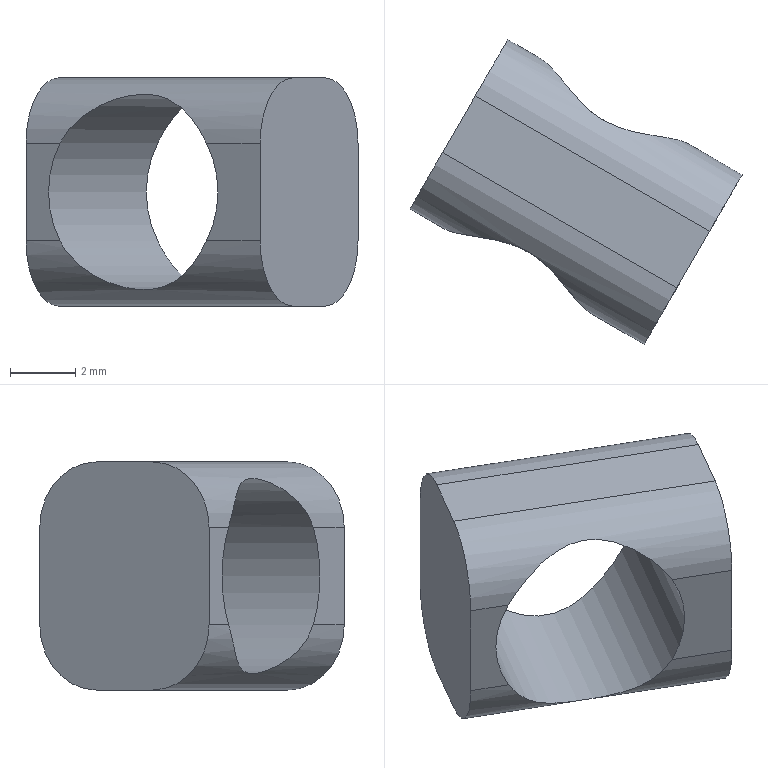Part | STEP file | 1 solid | 13 faces | box 10.188 x 9.346 x 7 mm | volume 153.66 mm3 | plane 8 | cylinder 5 | commonest cylinder face diameters 4 x4 6 x1
STEP:
#1=CARTESIAN_POINT('',(39.484,-2.012,-6.75));
#2=VERTEX_POINT('',#1);
#3=CARTESIAN_POINT('',(40.484,-0.2795,-4.75));
#4=VERTEX_POINT('',#3);
#5=CARTESIAN_POINT('',(40.484,-0.2795,-6.75));
#6=DIRECTION('',(-0.866,0.5,0.));
#7=DIRECTION('',(-0.5,-0.866,0.));
#8=AXIS2_PLACEMENT_3D('',#5,#6,#7);
#9=CIRCLE('',#8,2.);
#10=EDGE_CURVE('',#2,#4,#9,.T.);
#11=ORIENTED_EDGE('',*,*,#10,.T.);
#12=CARTESIAN_POINT('',(41.484,1.453,-4.75));
#13=VERTEX_POINT('',#12);
#14=CARTESIAN_POINT('',(40.484,-0.2795,-4.75));
#15=DIRECTION('',(0.5,0.866,0.));
#16=VECTOR('',#15,1.);
#17=LINE('',#14,#16);
#18=EDGE_CURVE('',#4,#13,#17,.T.);
#19=ORIENTED_EDGE('',*,*,#18,.T.);
#20=CARTESIAN_POINT('',(42.484,3.185,-6.75));
#21=VERTEX_POINT('',#20);
#22=CARTESIAN_POINT('',(41.484,1.453,-6.75));
#23=DIRECTION('',(-0.866,0.5,0.));
#24=DIRECTION('',(0.,0.,1.));
#25=AXIS2_PLACEMENT_3D('',#22,#23,#24);
#26=CIRCLE('',#25,2.);
#27=EDGE_CURVE('',#13,#21,#26,.T.);
#28=ORIENTED_EDGE('',*,*,#27,.T.);
#29=CARTESIAN_POINT('',(42.484,3.185,-9.75));
#30=VERTEX_POINT('',#29);
#31=CARTESIAN_POINT('',(42.484,3.185,-6.75));
#32=DIRECTION('',(0.,0.,-1.));
#33=VECTOR('',#32,1.);
#34=LINE('',#31,#33);
#35=EDGE_CURVE('',#21,#30,#34,.T.);
#36=ORIENTED_EDGE('',*,*,#35,.T.);
#37=CARTESIAN_POINT('',(41.484,1.453,-11.75));
#38=VERTEX_POINT('',#37);
#39=CARTESIAN_POINT('',(41.484,1.453,-9.75));
#40=DIRECTION('',(-0.866,0.5,0.));
#41=DIRECTION('',(0.5,0.866,0.));
#42=AXIS2_PLACEMENT_3D('',#39,#40,#41);
#43=CIRCLE('',#42,2.);
#44=EDGE_CURVE('',#30,#38,#43,.T.);
#45=ORIENTED_EDGE('',*,*,#44,.T.);
#46=CARTESIAN_POINT('',(40.484,-0.2795,-11.75));
#47=VERTEX_POINT('',#46);
#48=CARTESIAN_POINT('',(41.484,1.453,-11.75));
#49=DIRECTION('',(-0.5,-0.866,0.));
#50=VECTOR('',#49,1.);
#51=LINE('',#48,#50);
#52=EDGE_CURVE('',#38,#47,#51,.T.);
#53=ORIENTED_EDGE('',*,*,#52,.T.);
#54=CARTESIAN_POINT('',(39.484,-2.012,-9.75));
#55=VERTEX_POINT('',#54);
#56=CARTESIAN_POINT('',(40.484,-0.2795,-9.75));
#57=DIRECTION('',(-0.866,0.5,0.));
#58=DIRECTION('',(0.,0.,-1.));
#59=AXIS2_PLACEMENT_3D('',#56,#57,#58);
#60=CIRCLE('',#59,2.);
#61=EDGE_CURVE('',#47,#55,#60,.T.);
#62=ORIENTED_EDGE('',*,*,#61,.T.);
#63=CARTESIAN_POINT('',(39.484,-2.012,-9.75));
#64=DIRECTION('',(0.,0.,1.));
#65=VECTOR('',#64,1.);
#66=LINE('',#63,#65);
#67=EDGE_CURVE('',#55,#2,#66,.T.);
#68=ORIENTED_EDGE('',*,*,#67,.T.);
#69=EDGE_LOOP('',(#11,#19,#28,#36,#45,#53,#62,#68));
#70=FACE_BOUND('',#69,.T.);
#71=CARTESIAN_POINT('',(40.984,0.5865,-8.25));
#72=DIRECTION('',(0.866,-0.5,0.));
#73=DIRECTION('',(0.,0.,-1.));
#74=AXIS2_PLACEMENT_3D('',#71,#72,#73);
#75=PLANE('',#74);
#76=ADVANCED_FACE('',(#70),#75,.F.);
#77=ORIENTED_EDGE('',*,*,#67,.F.);
#78=CARTESIAN_POINT('',(40.525,-2.613,-9.75));
#79=VERTEX_POINT('',#78);
#80=CARTESIAN_POINT('',(40.525,-2.613,-9.75));
#81=DIRECTION('',(-0.866,0.5,0.));
#82=VECTOR('',#81,1.);
#83=LINE('',#80,#82);
#84=EDGE_CURVE('',#79,#55,#83,.T.);
#85=ORIENTED_EDGE('',*,*,#84,.F.);
#86=CARTESIAN_POINT('',(40.525,-2.613,-6.75));
#87=VERTEX_POINT('',#86);
#88=CARTESIAN_POINT('',(42.775,-3.912,-8.25));
#89=DIRECTION('',(0.5,0.866,0.));
#90=DIRECTION('',(-0.75,0.433,-0.5));
#91=AXIS2_PLACEMENT_3D('',#88,#89,#90);
#92=CIRCLE('',#91,3.);
#93=EDGE_CURVE('',#79,#87,#92,.T.);
#94=ORIENTED_EDGE('',*,*,#93,.T.);
#95=CARTESIAN_POINT('',(39.484,-2.012,-6.75));
#96=DIRECTION('',(0.866,-0.5,0.));
#97=VECTOR('',#96,1.);
#98=LINE('',#95,#97);
#99=EDGE_CURVE('',#2,#87,#98,.T.);
#100=ORIENTED_EDGE('',*,*,#99,.F.);
#101=EDGE_LOOP('',(#77,#85,#94,#100));
#102=FACE_BOUND('',#101,.T.);
#103=CARTESIAN_POINT('',(39.484,-2.012,-6.75));
#104=DIRECTION('',(-0.5,-0.866,0.));
#105=DIRECTION('',(-0.866,0.5,0.));
#106=AXIS2_PLACEMENT_3D('',#103,#104,#105);
#107=PLANE('',#106);
#108=ADVANCED_FACE('',(#102),#107,.T.);
#109=CARTESIAN_POINT('',(47.672,-4.429,-4.75));
#110=VERTEX_POINT('',#109);
#111=CARTESIAN_POINT('',(46.672,-6.162,-6.75));
#112=VERTEX_POINT('',#111);
#113=CARTESIAN_POINT('',(47.672,-4.429,-6.75));
#114=DIRECTION('',(0.866,-0.5,0.));
#115=DIRECTION('',(0.,0.,1.));
#116=AXIS2_PLACEMENT_3D('',#113,#114,#115);
#117=CIRCLE('',#116,2.);
#118=EDGE_CURVE('',#110,#112,#117,.T.);
#119=ORIENTED_EDGE('',*,*,#118,.F.);
#120=CARTESIAN_POINT('',(47.672,-4.429,-4.75));
#121=DIRECTION('',(-0.866,0.5,0.));
#122=VECTOR('',#121,1.);
#123=LINE('',#120,#122);
#124=EDGE_CURVE('',#110,#4,#123,.T.);
#125=ORIENTED_EDGE('',*,*,#124,.T.);
#126=ORIENTED_EDGE('',*,*,#10,.F.);
#127=ORIENTED_EDGE('',*,*,#99,.T.);
#128=CARTESIAN_POINT('',(43.114,-3.325,-5.25));
#129=VERTEX_POINT('',#128);
#130=CARTESIAN_POINT('',(40.525,-2.613,-6.75));
#131=CARTESIAN_POINT('',(40.535,-2.618,-6.731));
#132=CARTESIAN_POINT('',(40.555,-2.629,-6.692));
#133=CARTESIAN_POINT('',(40.587,-2.645,-6.635));
#134=CARTESIAN_POINT('',(40.621,-2.66,-6.578));
#135=CARTESIAN_POINT('',(40.657,-2.674,-6.523));
#136=CARTESIAN_POINT('',(40.694,-2.687,-6.469));
#137=CARTESIAN_POINT('',(40.733,-2.7,-6.415));
#138=CARTESIAN_POINT('',(40.774,-2.713,-6.363));
#139=CARTESIAN_POINT('',(40.816,-2.725,-6.311));
#140=CARTESIAN_POINT('',(40.861,-2.736,-6.26));
#141=CARTESIAN_POINT('',(40.907,-2.748,-6.209));
#142=CARTESIAN_POINT('',(40.956,-2.758,-6.16));
#143=CARTESIAN_POINT('',(41.006,-2.769,-6.111));
#144=CARTESIAN_POINT('',(41.058,-2.78,-6.062));
#145=CARTESIAN_POINT('',(41.112,-2.79,-6.015));
#146=CARTESIAN_POINT('',(41.167,-2.8,-5.968));
#147=CARTESIAN_POINT('',(41.224,-2.81,-5.923));
#148=CARTESIAN_POINT('',(41.282,-2.82,-5.879));
#149=CARTESIAN_POINT('',(41.342,-2.829,-5.837));
#150=CARTESIAN_POINT('',(41.402,-2.839,-5.796));
#151=CARTESIAN_POINT('',(41.462,-2.849,-5.756));
#152=CARTESIAN_POINT('',(41.523,-2.858,-5.719));
#153=CARTESIAN_POINT('',(41.584,-2.868,-5.683));
#154=CARTESIAN_POINT('',(41.645,-2.878,-5.649));
#155=CARTESIAN_POINT('',(41.706,-2.888,-5.617));
#156=CARTESIAN_POINT('',(41.766,-2.898,-5.586));
#157=CARTESIAN_POINT('',(41.826,-2.908,-5.557));
#158=CARTESIAN_POINT('',(41.885,-2.919,-5.53));
#159=CARTESIAN_POINT('',(41.943,-2.93,-5.505));
#160=CARTESIAN_POINT('',(42.,-2.94,-5.482));
#161=CARTESIAN_POINT('',(42.055,-2.952,-5.46));
#162=CARTESIAN_POINT('',(42.11,-2.963,-5.44));
#163=CARTESIAN_POINT('',(42.163,-2.975,-5.421));
#164=CARTESIAN_POINT('',(42.215,-2.986,-5.403));
#165=CARTESIAN_POINT('',(42.266,-2.999,-5.387));
#166=CARTESIAN_POINT('',(42.315,-3.011,-5.372));
#167=CARTESIAN_POINT('',(42.363,-3.023,-5.359));
#168=CARTESIAN_POINT('',(42.41,-3.036,-5.346));
#169=CARTESIAN_POINT('',(42.459,-3.05,-5.334));
#170=CARTESIAN_POINT('',(42.517,-3.068,-5.32));
#171=CARTESIAN_POINT('',(42.582,-3.089,-5.306));
#172=CARTESIAN_POINT('',(42.652,-3.113,-5.293));
#173=CARTESIAN_POINT('',(42.713,-3.135,-5.283));
#174=CARTESIAN_POINT('',(42.764,-3.155,-5.275));
#175=CARTESIAN_POINT('',(42.804,-3.172,-5.27));
#176=CARTESIAN_POINT('',(42.841,-3.188,-5.265));
#177=CARTESIAN_POINT('',(42.877,-3.204,-5.262));
#178=CARTESIAN_POINT('',(42.915,-3.221,-5.258));
#179=CARTESIAN_POINT('',(42.965,-3.245,-5.255));
#180=CARTESIAN_POINT('',(43.032,-3.279,-5.251));
#181=CARTESIAN_POINT('',(43.084,-3.308,-5.25));
#182=CARTESIAN_POINT('',(43.114,-3.325,-5.25));
#183=B_SPLINE_CURVE_WITH_KNOTS('',3,(#130,#131,#132,#133,#134,#135,#136,#137,#138,#139,#140,#141,#142,#143,#144,#145,#146,#147,#148,#149,#150,#151,#152,#153,#154,#155,#156,#157,#158,#159,#160,#161,#162,#163,#164,#165,#166,#167,#168,#169,#170,#171,#172,#173,#174,#175,#176,#177,#178,#179,#180,#181,#182),.UNSPECIFIED.,.F.,.F.,(4,1,1,1,1,1,1,1,1,1,1,1,1,1,1,1,1,1,1,1,1,1,1,1,1,1,1,1,1,1,1,1,1,1,1,1,1,1,1,1,1,1,1,1,1,1,1,1,1,1,4),(0.,0.0231,0.04593,0.06852,0.09084,0.113,0.135,0.1569,0.1787,0.2006,0.2226,0.2445,0.2666,0.2887,0.3109,0.3331,0.3552,0.3772,0.3991,0.4208,0.4421,0.4633,0.4841,0.5046,0.5247,0.5448,0.5644,0.5836,0.6023,0.6207,0.6386,0.6562,0.6733,0.6903,0.7067,0.7228,0.7383,0.7536,0.7698,0.7872,0.8115,0.8354,0.8588,0.8745,0.8885,0.901,0.9134,0.9272,0.9423,0.967,1.),.UNSPECIFIED.);
#184=EDGE_CURVE('',#87,#129,#183,.T.);
#185=ORIENTED_EDGE('',*,*,#184,.T.);
#186=CARTESIAN_POINT('',(45.025,-5.211,-6.75));
#187=VERTEX_POINT('',#186);
#188=CARTESIAN_POINT('',(45.025,-5.211,-6.75));
#189=CARTESIAN_POINT('',(45.015,-5.205,-6.731));
#190=CARTESIAN_POINT('',(44.996,-5.193,-6.692));
#191=CARTESIAN_POINT('',(44.966,-5.173,-6.635));
#192=CARTESIAN_POINT('',(44.937,-5.152,-6.579));
#193=CARTESIAN_POINT('',(44.907,-5.128,-6.524));
#194=CARTESIAN_POINT('',(44.876,-5.102,-6.47));
#195=CARTESIAN_POINT('',(44.845,-5.075,-6.416));
#196=CARTESIAN_POINT('',(44.814,-5.046,-6.364));
#197=CARTESIAN_POINT('',(44.782,-5.015,-6.312));
#198=CARTESIAN_POINT('',(44.75,-4.982,-6.26));
#199=CARTESIAN_POINT('',(44.717,-4.947,-6.21));
#200=CARTESIAN_POINT('',(44.684,-4.911,-6.16));
#201=CARTESIAN_POINT('',(44.65,-4.873,-6.111));
#202=CARTESIAN_POINT('',(44.615,-4.834,-6.063));
#203=CARTESIAN_POINT('',(44.579,-4.792,-6.016));
#204=CARTESIAN_POINT('',(44.543,-4.75,-5.97));
#205=CARTESIAN_POINT('',(44.506,-4.706,-5.925));
#206=CARTESIAN_POINT('',(44.469,-4.66,-5.881));
#207=CARTESIAN_POINT('',(44.431,-4.614,-5.839));
#208=CARTESIAN_POINT('',(44.393,-4.567,-5.798));
#209=CARTESIAN_POINT('',(44.354,-4.52,-5.759));
#210=CARTESIAN_POINT('',(44.316,-4.473,-5.721));
#211=CARTESIAN_POINT('',(44.277,-4.425,-5.686));
#212=CARTESIAN_POINT('',(44.238,-4.377,-5.652));
#213=CARTESIAN_POINT('',(44.2,-4.33,-5.62));
#214=CARTESIAN_POINT('',(44.161,-4.283,-5.589));
#215=CARTESIAN_POINT('',(44.122,-4.237,-5.56));
#216=CARTESIAN_POINT('',(44.084,-4.191,-5.534));
#217=CARTESIAN_POINT('',(44.046,-4.147,-5.508));
#218=CARTESIAN_POINT('',(44.009,-4.103,-5.485));
#219=CARTESIAN_POINT('',(43.972,-4.061,-5.463));
#220=CARTESIAN_POINT('',(43.935,-4.02,-5.443));
#221=CARTESIAN_POINT('',(43.898,-3.98,-5.424));
#222=CARTESIAN_POINT('',(43.862,-3.941,-5.406));
#223=CARTESIAN_POINT('',(43.827,-3.903,-5.39));
#224=CARTESIAN_POINT('',(43.792,-3.867,-5.375));
#225=CARTESIAN_POINT('',(43.757,-3.831,-5.361));
#226=CARTESIAN_POINT('',(43.723,-3.798,-5.349));
#227=CARTESIAN_POINT('',(43.69,-3.765,-5.337));
#228=CARTESIAN_POINT('',(43.657,-3.734,-5.327));
#229=CARTESIAN_POINT('',(43.624,-3.704,-5.317));
#230=CARTESIAN_POINT('',(43.591,-3.674,-5.308));
#231=CARTESIAN_POINT('',(43.556,-3.643,-5.299));
#232=CARTESIAN_POINT('',(43.511,-3.604,-5.289));
#233=CARTESIAN_POINT('',(43.449,-3.554,-5.277));
#234=CARTESIAN_POINT('',(43.368,-3.491,-5.265));
#235=CARTESIAN_POINT('',(43.278,-3.427,-5.256));
#236=CARTESIAN_POINT('',(43.192,-3.371,-5.251));
#237=CARTESIAN_POINT('',(43.138,-3.339,-5.25));
#238=CARTESIAN_POINT('',(43.114,-3.325,-5.25));
#239=B_SPLINE_CURVE_WITH_KNOTS('',3,(#188,#189,#190,#191,#192,#193,#194,#195,#196,#197,#198,#199,#200,#201,#202,#203,#204,#205,#206,#207,#208,#209,#210,#211,#212,#213,#214,#215,#216,#217,#218,#219,#220,#221,#222,#223,#224,#225,#226,#227,#228,#229,#230,#231,#232,#233,#234,#235,#236,#237,#238),.UNSPECIFIED.,.F.,.F.,(4,1,1,1,1,1,1,1,1,1,1,1,1,1,1,1,1,1,1,1,1,1,1,1,1,1,1,1,1,1,1,1,1,1,1,1,1,1,1,1,1,1,1,1,1,1,1,1,4),(0.,0.02202,0.04388,0.06559,0.08716,0.1087,0.1301,0.1515,0.1729,0.1943,0.2157,0.2372,0.2588,0.2805,0.3022,0.324,0.3457,0.3674,0.389,0.4104,0.4316,0.4526,0.4733,0.4938,0.5139,0.5339,0.5535,0.5727,0.5914,0.6099,0.6278,0.6454,0.6625,0.6796,0.6961,0.7122,0.7279,0.7434,0.7583,0.773,0.7872,0.8014,0.8167,0.8333,0.8599,0.8951,0.9359,0.9708,1.),.UNSPECIFIED.);
#240=EDGE_CURVE('',#187,#129,#239,.T.);
#241=ORIENTED_EDGE('',*,*,#240,.F.);
#242=CARTESIAN_POINT('',(45.025,-5.211,-6.75));
#243=DIRECTION('',(0.866,-0.5,0.));
#244=VECTOR('',#243,1.);
#245=LINE('',#242,#244);
#246=EDGE_CURVE('',#187,#112,#245,.T.);
#247=ORIENTED_EDGE('',*,*,#246,.T.);
#248=EDGE_LOOP('',(#119,#125,#126,#127,#185,#241,#247));
#249=FACE_BOUND('',#248,.T.);
#250=CARTESIAN_POINT('',(40.484,-0.2795,-6.75));
#251=DIRECTION('',(-0.866,0.5,0.));
#252=DIRECTION('',(0.,0.,-1.));
#253=AXIS2_PLACEMENT_3D('',#250,#251,#252);
#254=CYLINDRICAL_SURFACE('',#253,2.);
#255=ADVANCED_FACE('',(#249),#254,.T.);
#256=CARTESIAN_POINT('',(46.672,-6.162,-9.75));
#257=VERTEX_POINT('',#256);
#258=CARTESIAN_POINT('',(46.672,-6.162,-9.75));
#259=DIRECTION('',(0.,0.,1.));
#260=VECTOR('',#259,1.);
#261=LINE('',#258,#260);
#262=EDGE_CURVE('',#257,#112,#261,.T.);
#263=ORIENTED_EDGE('',*,*,#262,.T.);
#264=ORIENTED_EDGE('',*,*,#246,.F.);
#265=CARTESIAN_POINT('',(45.025,-5.211,-9.75));
#266=VERTEX_POINT('',#265);
#267=CARTESIAN_POINT('',(42.775,-3.912,-8.25));
#268=DIRECTION('',(0.5,0.866,0.));
#269=DIRECTION('',(0.75,-0.433,0.5));
#270=AXIS2_PLACEMENT_3D('',#267,#268,#269);
#271=CIRCLE('',#270,3.);
#272=EDGE_CURVE('',#187,#266,#271,.T.);
#273=ORIENTED_EDGE('',*,*,#272,.T.);
#274=CARTESIAN_POINT('',(46.672,-6.162,-9.75));
#275=DIRECTION('',(-0.866,0.5,0.));
#276=VECTOR('',#275,1.);
#277=LINE('',#274,#276);
#278=EDGE_CURVE('',#257,#266,#277,.T.);
#279=ORIENTED_EDGE('',*,*,#278,.F.);
#280=EDGE_LOOP('',(#263,#264,#273,#279));
#281=FACE_BOUND('',#280,.T.);
#282=CARTESIAN_POINT('',(39.484,-2.012,-6.75));
#283=DIRECTION('',(-0.5,-0.866,0.));
#284=DIRECTION('',(-0.866,0.5,0.));
#285=AXIS2_PLACEMENT_3D('',#282,#283,#284);
#286=PLANE('',#285);
#287=ADVANCED_FACE('',(#281),#286,.T.);
#288=ORIENTED_EDGE('',*,*,#84,.T.);
#289=ORIENTED_EDGE('',*,*,#61,.F.);
#290=CARTESIAN_POINT('',(47.672,-4.429,-11.75));
#291=VERTEX_POINT('',#290);
#292=CARTESIAN_POINT('',(40.484,-0.2795,-11.75));
#293=DIRECTION('',(0.866,-0.5,0.));
#294=VECTOR('',#293,1.);
#295=LINE('',#292,#294);
#296=EDGE_CURVE('',#47,#291,#295,.T.);
#297=ORIENTED_EDGE('',*,*,#296,.T.);
#298=CARTESIAN_POINT('',(47.672,-4.429,-9.75));
#299=DIRECTION('',(0.866,-0.5,0.));
#300=DIRECTION('',(-0.5,-0.866,0.));
#301=AXIS2_PLACEMENT_3D('',#298,#299,#300);
#302=CIRCLE('',#301,2.);
#303=EDGE_CURVE('',#257,#291,#302,.T.);
#304=ORIENTED_EDGE('',*,*,#303,.F.);
#305=ORIENTED_EDGE('',*,*,#278,.T.);
#306=CARTESIAN_POINT('',(45.025,-5.211,-9.75));
#307=CARTESIAN_POINT('',(45.008,-5.201,-9.784));
#308=CARTESIAN_POINT('',(44.978,-5.182,-9.843));
#309=CARTESIAN_POINT('',(44.937,-5.152,-9.92));
#310=CARTESIAN_POINT('',(44.902,-5.124,-9.984));
#311=CARTESIAN_POINT('',(44.871,-5.097,-10.04));
#312=CARTESIAN_POINT('',(44.839,-5.069,-10.095));
#313=CARTESIAN_POINT('',(44.806,-5.038,-10.149));
#314=CARTESIAN_POINT('',(44.774,-5.006,-10.203));
#315=CARTESIAN_POINT('',(44.74,-4.972,-10.255));
#316=CARTESIAN_POINT('',(44.707,-4.936,-10.306));
#317=CARTESIAN_POINT('',(44.673,-4.899,-10.355));
#318=CARTESIAN_POINT('',(44.639,-4.861,-10.404));
#319=CARTESIAN_POINT('',(44.602,-4.819,-10.453));
#320=CARTESIAN_POINT('',(44.563,-4.774,-10.505));
#321=CARTESIAN_POINT('',(44.518,-4.72,-10.561));
#322=CARTESIAN_POINT('',(44.466,-4.657,-10.622));
#323=CARTESIAN_POINT('',(44.407,-4.585,-10.687));
#324=CARTESIAN_POINT('',(44.345,-4.508,-10.751));
#325=CARTESIAN_POINT('',(44.28,-4.428,-10.812));
#326=CARTESIAN_POINT('',(44.217,-4.351,-10.867));
#327=CARTESIAN_POINT('',(44.158,-4.279,-10.913));
#328=CARTESIAN_POINT('',(44.104,-4.215,-10.953));
#329=CARTESIAN_POINT('',(44.056,-4.158,-10.985));
#330=CARTESIAN_POINT('',(44.011,-4.105,-11.014));
#331=CARTESIAN_POINT('',(43.966,-4.055,-11.04));
#332=CARTESIAN_POINT('',(43.922,-4.005,-11.064));
#333=CARTESIAN_POINT('',(43.877,-3.956,-11.087));
#334=CARTESIAN_POINT('',(43.831,-3.908,-11.108));
#335=CARTESIAN_POINT('',(43.781,-3.855,-11.129));
#336=CARTESIAN_POINT('',(43.726,-3.8,-11.151));
#337=CARTESIAN_POINT('',(43.665,-3.741,-11.171));
#338=CARTESIAN_POINT('',(43.61,-3.69,-11.187));
#339=CARTESIAN_POINT('',(43.56,-3.646,-11.2));
#340=CARTESIAN_POINT('',(43.516,-3.609,-11.21));
#341=CARTESIAN_POINT('',(43.473,-3.573,-11.218));
#342=CARTESIAN_POINT('',(43.43,-3.538,-11.226));
#343=CARTESIAN_POINT('',(43.387,-3.506,-11.232));
#344=CARTESIAN_POINT('',(43.345,-3.475,-11.237));
#345=CARTESIAN_POINT('',(43.304,-3.446,-11.242));
#346=CARTESIAN_POINT('',(43.264,-3.419,-11.245));
#347=CARTESIAN_POINT('',(43.225,-3.393,-11.247));
#348=CARTESIAN_POINT('',(43.187,-3.369,-11.249));
#349=CARTESIAN_POINT('',(43.15,-3.346,-11.25));
#350=CARTESIAN_POINT('',(43.125,-3.332,-11.25));
#351=CARTESIAN_POINT('',(43.101,-3.318,-11.25));
#352=CARTESIAN_POINT('',(43.077,-3.304,-11.25));
#353=CARTESIAN_POINT('',(43.042,-3.285,-11.249));
#354=CARTESIAN_POINT('',(43.007,-3.267,-11.248));
#355=CARTESIAN_POINT('',(42.973,-3.249,-11.246));
#356=CARTESIAN_POINT('',(42.939,-3.233,-11.244));
#357=CARTESIAN_POINT('',(42.906,-3.217,-11.241));
#358=CARTESIAN_POINT('',(42.873,-3.202,-11.238));
#359=CARTESIAN_POINT('',(42.84,-3.187,-11.234));
#360=CARTESIAN_POINT('',(42.807,-3.173,-11.231));
#361=CARTESIAN_POINT('',(42.773,-3.159,-11.226));
#362=CARTESIAN_POINT('',(42.739,-3.146,-11.221));
#363=CARTESIAN_POINT('',(42.703,-3.132,-11.216));
#364=CARTESIAN_POINT('',(42.663,-3.117,-11.209));
#365=CARTESIAN_POINT('',(42.619,-3.101,-11.201));
#366=CARTESIAN_POINT('',(42.57,-3.085,-11.191));
#367=CARTESIAN_POINT('',(42.518,-3.068,-11.18));
#368=CARTESIAN_POINT('',(42.466,-3.052,-11.168));
#369=CARTESIAN_POINT('',(42.413,-3.037,-11.155));
#370=CARTESIAN_POINT('',(42.362,-3.023,-11.141));
#371=CARTESIAN_POINT('',(42.314,-3.011,-11.127));
#372=CARTESIAN_POINT('',(42.268,-2.999,-11.113));
#373=CARTESIAN_POINT('',(42.222,-2.988,-11.099));
#374=CARTESIAN_POINT('',(42.176,-2.977,-11.084));
#375=CARTESIAN_POINT('',(42.128,-2.967,-11.067));
#376=CARTESIAN_POINT('',(42.08,-2.957,-11.049));
#377=CARTESIAN_POINT('',(42.03,-2.946,-11.03));
#378=CARTESIAN_POINT('',(41.979,-2.936,-11.01));
#379=CARTESIAN_POINT('',(41.927,-2.927,-10.988));
#380=CARTESIAN_POINT('',(41.874,-2.917,-10.964));
#381=CARTESIAN_POINT('',(41.818,-2.907,-10.939));
#382=CARTESIAN_POINT('',(41.757,-2.896,-10.909));
#383=CARTESIAN_POINT('',(41.681,-2.884,-10.871));
#384=CARTESIAN_POINT('',(41.593,-2.869,-10.822));
#385=CARTESIAN_POINT('',(41.495,-2.854,-10.765));
#386=CARTESIAN_POINT('',(41.409,-2.84,-10.71));
#387=CARTESIAN_POINT('',(41.336,-2.828,-10.66));
#388=CARTESIAN_POINT('',(41.279,-2.819,-10.618));
#389=CARTESIAN_POINT('',(41.226,-2.81,-10.578));
#390=CARTESIAN_POINT('',(41.177,-2.802,-10.539));
#391=CARTESIAN_POINT('',(41.129,-2.793,-10.5));
#392=CARTESIAN_POINT('',(41.082,-2.784,-10.459));
#393=CARTESIAN_POINT('',(41.037,-2.775,-10.418));
#394=CARTESIAN_POINT('',(40.993,-2.766,-10.377));
#395=CARTESIAN_POINT('',(40.95,-2.757,-10.335));
#396=CARTESIAN_POINT('',(40.91,-2.748,-10.293));
#397=CARTESIAN_POINT('',(40.87,-2.739,-10.251));
#398=CARTESIAN_POINT('',(40.833,-2.729,-10.208));
#399=CARTESIAN_POINT('',(40.798,-2.719,-10.166));
#400=CARTESIAN_POINT('',(40.764,-2.71,-10.124));
#401=CARTESIAN_POINT('',(40.731,-2.7,-10.082));
#402=CARTESIAN_POINT('',(40.701,-2.69,-10.04));
#403=CARTESIAN_POINT('',(40.671,-2.679,-9.999));
#404=CARTESIAN_POINT('',(40.644,-2.669,-9.957));
#405=CARTESIAN_POINT('',(40.617,-2.658,-9.915));
#406=CARTESIAN_POINT('',(40.592,-2.647,-9.874));
#407=CARTESIAN_POINT('',(40.569,-2.636,-9.833));
#408=CARTESIAN_POINT('',(40.546,-2.624,-9.792));
#409=CARTESIAN_POINT('',(40.532,-2.617,-9.764));
#410=CARTESIAN_POINT('',(40.525,-2.613,-9.75));
#411=B_SPLINE_CURVE_WITH_KNOTS('',3,(#306,#307,#308,#309,#310,#311,#312,#313,#314,#315,#316,#317,#318,#319,#320,#321,#322,#323,#324,#325,#326,#327,#328,#329,#330,#331,#332,#333,#334,#335,#336,#337,#338,#339,#340,#341,#342,#343,#344,#345,#346,#347,#348,#349,#350,#351,#352,#353,#354,#355,#356,#357,#358,#359,#360,#361,#362,#363,#364,#365,#366,#367,#368,#369,#370,#371,#372,#373,#374,#375,#376,#377,#378,#379,#380,#381,#382,#383,#384,#385,#386,#387,#388,#389,#390,#391,#392,#393,#394,#395,#396,#397,#398,#399,#400,#401,#402,#403,#404,#405,#406,#407,#408,#409,#410),.UNSPECIFIED.,.F.,.F.,(4,1,1,1,1,1,1,1,1,1,1,1,1,1,1,1,1,1,1,1,1,1,1,1,1,1,1,1,1,1,1,1,1,1,1,1,1,1,1,1,1,1,1,1,1,1,1,1,1,1,1,1,1,1,1,1,1,1,1,1,1,1,1,1,1,1,1,1,1,1,1,1,1,1,1,1,1,1,1,1,1,1,1,1,1,1,1,1,1,1,1,1,1,1,1,1,1,1,1,1,1,1,4),(0.,0.01788,0.03215,0.04291,0.05374,0.06463,0.07554,0.08646,0.09738,0.1083,0.1193,0.1302,0.1412,0.1535,0.1671,0.1832,0.2007,0.2195,0.2384,0.2561,0.2725,0.2865,0.2991,0.3103,0.3215,0.3325,0.3435,0.3542,0.3648,0.3785,0.3919,0.4049,0.4142,0.4233,0.4322,0.4409,0.4492,0.4573,0.4651,0.4727,0.4799,0.4869,0.4936,0.5,0.5002,0.5066,0.5128,0.5188,0.5248,0.5306,0.5363,0.5419,0.5475,0.5531,0.5588,0.5646,0.5704,0.577,0.5844,0.5927,0.6013,0.6101,0.619,0.6275,0.6354,0.6429,0.6505,0.6582,0.6661,0.6743,0.6827,0.6914,0.7003,0.7095,0.7187,0.7292,0.7411,0.7587,0.7765,0.7943,0.8066,0.8177,0.8277,0.8375,0.8473,0.8569,0.8665,0.876,0.8853,0.8945,0.9035,0.9124,0.9211,0.9296,0.9379,0.9461,0.9542,0.9621,0.9699,0.9776,0.9851,0.9926,1.),.UNSPECIFIED.);
#412=EDGE_CURVE('',#266,#79,#411,.T.);
#413=ORIENTED_EDGE('',*,*,#412,.T.);
#414=EDGE_LOOP('',(#288,#289,#297,#304,#305,#413));
#415=FACE_BOUND('',#414,.T.);
#416=CARTESIAN_POINT('',(40.484,-0.2795,-9.75));
#417=DIRECTION('',(-0.866,0.5,0.));
#418=DIRECTION('',(0.,0.,-1.));
#419=AXIS2_PLACEMENT_3D('',#416,#417,#418);
#420=CYLINDRICAL_SURFACE('',#419,2.);
#421=ADVANCED_FACE('',(#415),#420,.T.);
#422=CARTESIAN_POINT('',(48.025,-0.01443,-9.75));
#423=VERTEX_POINT('',#422);
#424=CARTESIAN_POINT('',(48.025,-0.01443,-6.75));
#425=VERTEX_POINT('',#424);
#426=CARTESIAN_POINT('',(45.775,1.285,-8.25));
#427=DIRECTION('',(-0.5,-0.866,0.));
#428=DIRECTION('',(0.75,-0.433,-0.5));
#429=AXIS2_PLACEMENT_3D('',#426,#427,#428);
#430=CIRCLE('',#429,3.);
#431=EDGE_CURVE('',#423,#425,#430,.T.);
#432=ORIENTED_EDGE('',*,*,#431,.F.);
#433=CARTESIAN_POINT('',(43.525,2.584,-9.75));
#434=VERTEX_POINT('',#433);
#435=CARTESIAN_POINT('',(48.025,-0.01443,-9.75));
#436=CARTESIAN_POINT('',(48.015,-0.008652,-9.77));
#437=CARTESIAN_POINT('',(47.994,0.002583,-9.81));
#438=CARTESIAN_POINT('',(47.961,0.01856,-9.868));
#439=CARTESIAN_POINT('',(47.927,0.03375,-9.926));
#440=CARTESIAN_POINT('',(47.89,0.04825,-9.982));
#441=CARTESIAN_POINT('',(47.851,0.06213,-10.038));
#442=CARTESIAN_POINT('',(47.811,0.07542,-10.093));
#443=CARTESIAN_POINT('',(47.768,0.08814,-10.147));
#444=CARTESIAN_POINT('',(47.724,0.1003,-10.2));
#445=CARTESIAN_POINT('',(47.679,0.112,-10.252));
#446=CARTESIAN_POINT('',(47.631,0.1232,-10.302));
#447=CARTESIAN_POINT('',(47.583,0.1341,-10.352));
#448=CARTESIAN_POINT('',(47.533,0.1446,-10.4));
#449=CARTESIAN_POINT('',(47.479,0.1552,-10.45));
#450=CARTESIAN_POINT('',(47.42,0.1662,-10.501));
#451=CARTESIAN_POINT('',(47.351,0.1786,-10.558));
#452=CARTESIAN_POINT('',(47.271,0.1921,-10.619));
#453=CARTESIAN_POINT('',(47.18,0.207,-10.683));
#454=CARTESIAN_POINT('',(47.082,0.2226,-10.748));
#455=CARTESIAN_POINT('',(46.981,0.2386,-10.809));
#456=CARTESIAN_POINT('',(46.883,0.2545,-10.863));
#457=CARTESIAN_POINT('',(46.792,0.2696,-10.91));
#458=CARTESIAN_POINT('',(46.71,0.2839,-10.949));
#459=CARTESIAN_POINT('',(46.637,0.2971,-10.982));
#460=CARTESIAN_POINT('',(46.568,0.31,-11.011));
#461=CARTESIAN_POINT('',(46.502,0.323,-11.037));
#462=CARTESIAN_POINT('',(46.437,0.3367,-11.062));
#463=CARTESIAN_POINT('',(46.372,0.3509,-11.084));
#464=CARTESIAN_POINT('',(46.308,0.3659,-11.106));
#465=CARTESIAN_POINT('',(46.237,0.3832,-11.127));
#466=CARTESIAN_POINT('',(46.161,0.4034,-11.149));
#467=CARTESIAN_POINT('',(46.079,0.4266,-11.169));
#468=CARTESIAN_POINT('',(46.005,0.4497,-11.186));
#469=CARTESIAN_POINT('',(45.935,0.473,-11.2));
#470=CARTESIAN_POINT('',(45.868,0.4969,-11.213));
#471=CARTESIAN_POINT('',(45.798,0.5234,-11.223));
#472=CARTESIAN_POINT('',(45.73,0.5517,-11.232));
#473=CARTESIAN_POINT('',(45.663,0.5812,-11.239));
#474=CARTESIAN_POINT('',(45.599,0.6115,-11.245));
#475=CARTESIAN_POINT('',(45.537,0.6425,-11.248));
#476=CARTESIAN_POINT('',(45.484,0.6714,-11.25));
#477=CARTESIAN_POINT('',(45.44,0.6961,-11.25));
#478=CARTESIAN_POINT('',(45.391,0.7245,-11.25));
#479=CARTESIAN_POINT('',(45.334,0.7601,-11.248));
#480=CARTESIAN_POINT('',(45.272,0.8011,-11.244));
#481=CARTESIAN_POINT('',(45.22,0.8373,-11.239));
#482=CARTESIAN_POINT('',(45.179,0.8674,-11.234));
#483=CARTESIAN_POINT('',(45.14,0.8963,-11.229));
#484=CARTESIAN_POINT('',(45.102,0.9261,-11.223));
#485=CARTESIAN_POINT('',(45.061,0.9593,-11.215));
#486=CARTESIAN_POINT('',(45.009,1.002,-11.205));
#487=CARTESIAN_POINT('',(44.949,1.055,-11.19));
#488=CARTESIAN_POINT('',(44.882,1.117,-11.17));
#489=CARTESIAN_POINT('',(44.823,1.174,-11.15));
#490=CARTESIAN_POINT('',(44.772,1.225,-11.131));
#491=CARTESIAN_POINT('',(44.73,1.268,-11.113));
#492=CARTESIAN_POINT('',(44.691,1.31,-11.095));
#493=CARTESIAN_POINT('',(44.653,1.351,-11.077));
#494=CARTESIAN_POINT('',(44.615,1.393,-11.057));
#495=CARTESIAN_POINT('',(44.576,1.436,-11.036));
#496=CARTESIAN_POINT('',(44.538,1.48,-11.013));
#497=CARTESIAN_POINT('',(44.5,1.524,-10.989));
#498=CARTESIAN_POINT('',(44.462,1.568,-10.964));
#499=CARTESIAN_POINT('',(44.425,1.613,-10.938));
#500=CARTESIAN_POINT('',(44.388,1.657,-10.91));
#501=CARTESIAN_POINT('',(44.352,1.701,-10.881));
#502=CARTESIAN_POINT('',(44.316,1.745,-10.852));
#503=CARTESIAN_POINT('',(44.281,1.788,-10.821));
#504=CARTESIAN_POINT('',(44.246,1.831,-10.79));
#505=CARTESIAN_POINT('',(44.212,1.873,-10.758));
#506=CARTESIAN_POINT('',(44.178,1.914,-10.724));
#507=CARTESIAN_POINT('',(44.144,1.957,-10.688));
#508=CARTESIAN_POINT('',(44.109,1.999,-10.65));
#509=CARTESIAN_POINT('',(44.067,2.051,-10.603));
#510=CARTESIAN_POINT('',(44.012,2.117,-10.537));
#511=CARTESIAN_POINT('',(43.94,2.202,-10.444));
#512=CARTESIAN_POINT('',(43.865,2.286,-10.339));
#513=CARTESIAN_POINT('',(43.801,2.355,-10.241));
#514=CARTESIAN_POINT('',(43.755,2.4,-10.168));
#515=CARTESIAN_POINT('',(43.72,2.434,-10.109));
#516=CARTESIAN_POINT('',(43.689,2.462,-10.056));
#517=CARTESIAN_POINT('',(43.66,2.487,-10.006));
#518=CARTESIAN_POINT('',(43.637,2.506,-9.965));
#519=CARTESIAN_POINT('',(43.619,2.52,-9.932));
#520=CARTESIAN_POINT('',(43.603,2.532,-9.902));
#521=CARTESIAN_POINT('',(43.587,2.544,-9.871));
#522=CARTESIAN_POINT('',(43.571,2.555,-9.841));
#523=CARTESIAN_POINT('',(43.556,2.565,-9.811));
#524=CARTESIAN_POINT('',(43.54,2.575,-9.781));
#525=CARTESIAN_POINT('',(43.53,2.581,-9.76));
#526=CARTESIAN_POINT('',(43.525,2.584,-9.75));
#527=B_SPLINE_CURVE_WITH_KNOTS('',3,(#435,#436,#437,#438,#439,#440,#441,#442,#443,#444,#445,#446,#447,#448,#449,#450,#451,#452,#453,#454,#455,#456,#457,#458,#459,#460,#461,#462,#463,#464,#465,#466,#467,#468,#469,#470,#471,#472,#473,#474,#475,#476,#477,#478,#479,#480,#481,#482,#483,#484,#485,#486,#487,#488,#489,#490,#491,#492,#493,#494,#495,#496,#497,#498,#499,#500,#501,#502,#503,#504,#505,#506,#507,#508,#509,#510,#511,#512,#513,#514,#515,#516,#517,#518,#519,#520,#521,#522,#523,#524,#525,#526),.UNSPECIFIED.,.F.,.F.,(4,1,1,1,1,1,1,1,1,1,1,1,1,1,1,1,1,1,1,1,1,1,1,1,1,1,1,1,1,1,1,1,1,1,1,1,1,1,1,1,1,1,1,1,1,1,1,1,1,1,1,1,1,1,1,1,1,1,1,1,1,1,1,1,1,1,1,1,1,1,1,1,1,1,1,1,1,1,1,1,1,1,1,1,1,1,1,1,1,4),(0.,0.01066,0.02129,0.03192,0.04261,0.05337,0.06419,0.07503,0.08588,0.09674,0.1076,0.1185,0.1294,0.1404,0.1526,0.1661,0.1822,0.1997,0.2184,0.2372,0.2549,0.2713,0.2852,0.2978,0.309,0.3202,0.3312,0.3421,0.3529,0.3635,0.3773,0.3908,0.404,0.4144,0.4257,0.4376,0.4493,0.4605,0.4717,0.4823,0.4925,0.5,0.5056,0.5186,0.5314,0.5402,0.5481,0.5553,0.5626,0.5709,0.5801,0.5942,0.6086,0.6232,0.6336,0.6433,0.6524,0.6615,0.6708,0.6803,0.69,0.6998,0.7096,0.7195,0.7294,0.7393,0.7492,0.7591,0.7688,0.7785,0.7883,0.7983,0.8087,0.8194,0.8364,0.859,0.8869,0.9078,0.922,0.9321,0.9433,0.9536,0.9612,0.9668,0.9724,0.978,0.9835,0.9891,0.9945,1.),.UNSPECIFIED.);
#528=EDGE_CURVE('',#423,#434,#527,.T.);
#529=ORIENTED_EDGE('',*,*,#528,.T.);
#530=CARTESIAN_POINT('',(43.525,2.584,-6.75));
#531=VERTEX_POINT('',#530);
#532=CARTESIAN_POINT('',(45.775,1.285,-8.25));
#533=DIRECTION('',(-0.5,-0.866,0.));
#534=DIRECTION('',(-0.75,0.433,0.5));
#535=AXIS2_PLACEMENT_3D('',#532,#533,#534);
#536=CIRCLE('',#535,3.);
#537=EDGE_CURVE('',#531,#434,#536,.T.);
#538=ORIENTED_EDGE('',*,*,#537,.F.);
#539=CARTESIAN_POINT('',(45.436,0.6982,-5.25));
#540=VERTEX_POINT('',#539);
#541=CARTESIAN_POINT('',(43.525,2.584,-6.75));
#542=CARTESIAN_POINT('',(43.535,2.578,-6.731));
#543=CARTESIAN_POINT('',(43.554,2.566,-6.692));
#544=CARTESIAN_POINT('',(43.584,2.546,-6.635));
#545=CARTESIAN_POINT('',(43.613,2.525,-6.579));
#546=CARTESIAN_POINT('',(43.643,2.501,-6.524));
#547=CARTESIAN_POINT('',(43.674,2.475,-6.47));
#548=CARTESIAN_POINT('',(43.705,2.448,-6.416));
#549=CARTESIAN_POINT('',(43.736,2.419,-6.364));
#550=CARTESIAN_POINT('',(43.768,2.388,-6.312));
#551=CARTESIAN_POINT('',(43.8,2.355,-6.26));
#552=CARTESIAN_POINT('',(43.833,2.32,-6.21));
#553=CARTESIAN_POINT('',(43.866,2.284,-6.16));
#554=CARTESIAN_POINT('',(43.9,2.246,-6.111));
#555=CARTESIAN_POINT('',(43.935,2.207,-6.063));
#556=CARTESIAN_POINT('',(43.971,2.165,-6.016));
#557=CARTESIAN_POINT('',(44.007,2.123,-5.97));
#558=CARTESIAN_POINT('',(44.044,2.079,-5.925));
#559=CARTESIAN_POINT('',(44.081,2.033,-5.881));
#560=CARTESIAN_POINT('',(44.119,1.987,-5.839));
#561=CARTESIAN_POINT('',(44.157,1.94,-5.798));
#562=CARTESIAN_POINT('',(44.196,1.893,-5.759));
#563=CARTESIAN_POINT('',(44.234,1.846,-5.721));
#564=CARTESIAN_POINT('',(44.273,1.798,-5.686));
#565=CARTESIAN_POINT('',(44.311,1.75,-5.652));
#566=CARTESIAN_POINT('',(44.35,1.703,-5.62));
#567=CARTESIAN_POINT('',(44.389,1.656,-5.589));
#568=CARTESIAN_POINT('',(44.428,1.61,-5.56));
#569=CARTESIAN_POINT('',(44.466,1.564,-5.534));
#570=CARTESIAN_POINT('',(44.504,1.52,-5.508));
#571=CARTESIAN_POINT('',(44.541,1.476,-5.485));
#572=CARTESIAN_POINT('',(44.578,1.434,-5.463));
#573=CARTESIAN_POINT('',(44.615,1.393,-5.443));
#574=CARTESIAN_POINT('',(44.652,1.353,-5.424));
#575=CARTESIAN_POINT('',(44.688,1.314,-5.406));
#576=CARTESIAN_POINT('',(44.723,1.276,-5.39));
#577=CARTESIAN_POINT('',(44.758,1.24,-5.375));
#578=CARTESIAN_POINT('',(44.793,1.204,-5.361));
#579=CARTESIAN_POINT('',(44.827,1.171,-5.349));
#580=CARTESIAN_POINT('',(44.86,1.138,-5.337));
#581=CARTESIAN_POINT('',(44.893,1.107,-5.327));
#582=CARTESIAN_POINT('',(44.926,1.077,-5.317));
#583=CARTESIAN_POINT('',(44.959,1.047,-5.308));
#584=CARTESIAN_POINT('',(44.994,1.016,-5.299));
#585=CARTESIAN_POINT('',(45.039,0.977,-5.289));
#586=CARTESIAN_POINT('',(45.101,0.9268,-5.277));
#587=CARTESIAN_POINT('',(45.182,0.8641,-5.265));
#588=CARTESIAN_POINT('',(45.272,0.8005,-5.256));
#589=CARTESIAN_POINT('',(45.358,0.7444,-5.251));
#590=CARTESIAN_POINT('',(45.412,0.7124,-5.25));
#591=CARTESIAN_POINT('',(45.436,0.6982,-5.25));
#592=B_SPLINE_CURVE_WITH_KNOTS('',3,(#541,#542,#543,#544,#545,#546,#547,#548,#549,#550,#551,#552,#553,#554,#555,#556,#557,#558,#559,#560,#561,#562,#563,#564,#565,#566,#567,#568,#569,#570,#571,#572,#573,#574,#575,#576,#577,#578,#579,#580,#581,#582,#583,#584,#585,#586,#587,#588,#589,#590,#591),.UNSPECIFIED.,.F.,.F.,(4,1,1,1,1,1,1,1,1,1,1,1,1,1,1,1,1,1,1,1,1,1,1,1,1,1,1,1,1,1,1,1,1,1,1,1,1,1,1,1,1,1,1,1,1,1,1,1,4),(0.,0.02203,0.04388,0.06559,0.08717,0.1087,0.1301,0.1515,0.1729,0.1943,0.2158,0.2372,0.2588,0.2805,0.3022,0.324,0.3457,0.3674,0.389,0.4104,0.4316,0.4526,0.4733,0.4938,0.5139,0.5339,0.5535,0.5728,0.5915,0.6099,0.6278,0.6454,0.6626,0.6796,0.6961,0.7123,0.7279,0.7434,0.7583,0.773,0.7873,0.8014,0.8167,0.8333,0.8599,0.8951,0.9359,0.9709,1.),.UNSPECIFIED.);
#593=EDGE_CURVE('',#531,#540,#592,.T.);
#594=ORIENTED_EDGE('',*,*,#593,.T.);
#595=CARTESIAN_POINT('',(45.436,0.6982,-5.25));
#596=CARTESIAN_POINT('',(45.455,0.6874,-5.25));
#597=CARTESIAN_POINT('',(45.493,0.6661,-5.25));
#598=CARTESIAN_POINT('',(45.551,0.6355,-5.253));
#599=CARTESIAN_POINT('',(45.609,0.6063,-5.256));
#600=CARTESIAN_POINT('',(45.669,0.5784,-5.261));
#601=CARTESIAN_POINT('',(45.729,0.5518,-5.268));
#602=CARTESIAN_POINT('',(45.791,0.5264,-5.276));
#603=CARTESIAN_POINT('',(45.853,0.5023,-5.285));
#604=CARTESIAN_POINT('',(45.917,0.4793,-5.296));
#605=CARTESIAN_POINT('',(45.981,0.4574,-5.309));
#606=CARTESIAN_POINT('',(46.047,0.4366,-5.323));
#607=CARTESIAN_POINT('',(46.113,0.4169,-5.339));
#608=CARTESIAN_POINT('',(46.18,0.3981,-5.357));
#609=CARTESIAN_POINT('',(46.249,0.3803,-5.376));
#610=CARTESIAN_POINT('',(46.318,0.3635,-5.398));
#611=CARTESIAN_POINT('',(46.387,0.3475,-5.421));
#612=CARTESIAN_POINT('',(46.457,0.3324,-5.446));
#613=CARTESIAN_POINT('',(46.527,0.3181,-5.472));
#614=CARTESIAN_POINT('',(46.596,0.3046,-5.501));
#615=CARTESIAN_POINT('',(46.666,0.2917,-5.531));
#616=CARTESIAN_POINT('',(46.735,0.2795,-5.562));
#617=CARTESIAN_POINT('',(46.803,0.2679,-5.595));
#618=CARTESIAN_POINT('',(46.87,0.2567,-5.63));
#619=CARTESIAN_POINT('',(46.936,0.2459,-5.666));
#620=CARTESIAN_POINT('',(47.002,0.2354,-5.704));
#621=CARTESIAN_POINT('',(47.066,0.2252,-5.743));
#622=CARTESIAN_POINT('',(47.129,0.2152,-5.783));
#623=CARTESIAN_POINT('',(47.19,0.2054,-5.824));
#624=CARTESIAN_POINT('',(47.249,0.1957,-5.866));
#625=CARTESIAN_POINT('',(47.306,0.1861,-5.908));
#626=CARTESIAN_POINT('',(47.362,0.1766,-5.952));
#627=CARTESIAN_POINT('',(47.421,0.166,-6.));
#628=CARTESIAN_POINT('',(47.484,0.1543,-6.054));
#629=CARTESIAN_POINT('',(47.548,0.1415,-6.114));
#630=CARTESIAN_POINT('',(47.604,0.1295,-6.169));
#631=CARTESIAN_POINT('',(47.651,0.1185,-6.219));
#632=CARTESIAN_POINT('',(47.692,0.1086,-6.263));
#633=CARTESIAN_POINT('',(47.731,0.09854,-6.308));
#634=CARTESIAN_POINT('',(47.767,0.08838,-6.352));
#635=CARTESIAN_POINT('',(47.802,0.07804,-6.396));
#636=CARTESIAN_POINT('',(47.835,0.06749,-6.44));
#637=CARTESIAN_POINT('',(47.867,0.05668,-6.484));
#638=CARTESIAN_POINT('',(47.897,0.04563,-6.528));
#639=CARTESIAN_POINT('',(47.925,0.03431,-6.572));
#640=CARTESIAN_POINT('',(47.952,0.02268,-6.616));
#641=CARTESIAN_POINT('',(47.978,0.01071,-6.661));
#642=CARTESIAN_POINT('',(48.002,-0.001621,-6.705));
#643=CARTESIAN_POINT('',(48.018,-0.01011,-6.735));
#644=CARTESIAN_POINT('',(48.025,-0.01443,-6.75));
#645=B_SPLINE_CURVE_WITH_KNOTS('',3,(#595,#596,#597,#598,#599,#600,#601,#602,#603,#604,#605,#606,#607,#608,#609,#610,#611,#612,#613,#614,#615,#616,#617,#618,#619,#620,#621,#622,#623,#624,#625,#626,#627,#628,#629,#630,#631,#632,#633,#634,#635,#636,#637,#638,#639,#640,#641,#642,#643,#644),.UNSPECIFIED.,.F.,.F.,(4,1,1,1,1,1,1,1,1,1,1,1,1,1,1,1,1,1,1,1,1,1,1,1,1,1,1,1,1,1,1,1,1,1,1,1,1,1,1,1,1,1,1,1,1,1,1,4),(0.,0.02256,0.04491,0.06709,0.08916,0.1112,0.1332,0.1553,0.1773,0.1995,0.2217,0.244,0.2665,0.2891,0.3118,0.3347,0.3574,0.3802,0.4029,0.4256,0.4481,0.4705,0.4929,0.5152,0.5374,0.5595,0.5814,0.6033,0.6248,0.6461,0.6672,0.6881,0.7153,0.7422,0.7688,0.788,0.8071,0.8256,0.8439,0.8618,0.8796,0.8972,0.9146,0.9319,0.949,0.9661,0.983,1.),.UNSPECIFIED.);
#646=EDGE_CURVE('',#540,#425,#645,.T.);
#647=ORIENTED_EDGE('',*,*,#646,.T.);
#648=EDGE_LOOP('',(#432,#529,#538,#594,#647));
#649=FACE_BOUND('',#648,.T.);
#650=ORIENTED_EDGE('',*,*,#240,.T.);
#651=ORIENTED_EDGE('',*,*,#184,.F.);
#652=ORIENTED_EDGE('',*,*,#93,.F.);
#653=ORIENTED_EDGE('',*,*,#412,.F.);
#654=ORIENTED_EDGE('',*,*,#272,.F.);
#655=EDGE_LOOP('',(#650,#651,#652,#653,#654));
#656=FACE_BOUND('',#655,.T.);
#657=CARTESIAN_POINT('',(42.775,-3.912,-8.25));
#658=DIRECTION('',(-0.5,-0.866,0.));
#659=DIRECTION('',(0.,0.,1.));
#660=AXIS2_PLACEMENT_3D('',#657,#658,#659);
#661=CYLINDRICAL_SURFACE('',#660,3.);
#662=ADVANCED_FACE('',(#649,#656),#661,.F.);
#663=CARTESIAN_POINT('',(48.672,-2.697,-11.75));
#664=VERTEX_POINT('',#663);
#665=CARTESIAN_POINT('',(49.672,-0.9654,-9.75));
#666=VERTEX_POINT('',#665);
#667=CARTESIAN_POINT('',(48.672,-2.697,-9.75));
#668=DIRECTION('',(0.866,-0.5,0.));
#669=DIRECTION('',(0.,0.,-1.));
#670=AXIS2_PLACEMENT_3D('',#667,#668,#669);
#671=CIRCLE('',#670,2.);
#672=EDGE_CURVE('',#664,#666,#671,.T.);
#673=ORIENTED_EDGE('',*,*,#672,.F.);
#674=CARTESIAN_POINT('',(48.672,-2.697,-11.75));
#675=DIRECTION('',(-0.866,0.5,0.));
#676=VECTOR('',#675,1.);
#677=LINE('',#674,#676);
#678=EDGE_CURVE('',#664,#38,#677,.T.);
#679=ORIENTED_EDGE('',*,*,#678,.T.);
#680=ORIENTED_EDGE('',*,*,#44,.F.);
#681=CARTESIAN_POINT('',(42.484,3.185,-9.75));
#682=DIRECTION('',(0.866,-0.5,0.));
#683=VECTOR('',#682,1.);
#684=LINE('',#681,#683);
#685=EDGE_CURVE('',#30,#434,#684,.T.);
#686=ORIENTED_EDGE('',*,*,#685,.T.);
#687=ORIENTED_EDGE('',*,*,#528,.F.);
#688=CARTESIAN_POINT('',(48.025,-0.01443,-9.75));
#689=DIRECTION('',(0.866,-0.5,0.));
#690=VECTOR('',#689,1.);
#691=LINE('',#688,#690);
#692=EDGE_CURVE('',#423,#666,#691,.T.);
#693=ORIENTED_EDGE('',*,*,#692,.T.);
#694=EDGE_LOOP('',(#673,#679,#680,#686,#687,#693));
#695=FACE_BOUND('',#694,.T.);
#696=CARTESIAN_POINT('',(41.484,1.453,-9.75));
#697=DIRECTION('',(-0.866,0.5,0.));
#698=DIRECTION('',(0.,0.,-1.));
#699=AXIS2_PLACEMENT_3D('',#696,#697,#698);
#700=CYLINDRICAL_SURFACE('',#699,2.);
#701=ADVANCED_FACE('',(#695),#700,.T.);
#702=CARTESIAN_POINT('',(49.672,-0.9654,-6.75));
#703=VERTEX_POINT('',#702);
#704=CARTESIAN_POINT('',(49.672,-0.9654,-6.75));
#705=DIRECTION('',(0.,0.,-1.));
#706=VECTOR('',#705,1.);
#707=LINE('',#704,#706);
#708=EDGE_CURVE('',#703,#666,#707,.T.);
#709=ORIENTED_EDGE('',*,*,#708,.T.);
#710=ORIENTED_EDGE('',*,*,#692,.F.);
#711=ORIENTED_EDGE('',*,*,#431,.T.);
#712=CARTESIAN_POINT('',(49.672,-0.9654,-6.75));
#713=DIRECTION('',(-0.866,0.5,0.));
#714=VECTOR('',#713,1.);
#715=LINE('',#712,#714);
#716=EDGE_CURVE('',#703,#425,#715,.T.);
#717=ORIENTED_EDGE('',*,*,#716,.F.);
#718=EDGE_LOOP('',(#709,#710,#711,#717));
#719=FACE_BOUND('',#718,.T.);
#720=CARTESIAN_POINT('',(42.484,3.185,-9.75));
#721=DIRECTION('',(0.5,0.866,0.));
#722=DIRECTION('',(0.,0.,-1.));
#723=AXIS2_PLACEMENT_3D('',#720,#721,#722);
#724=PLANE('',#723);
#725=ADVANCED_FACE('',(#719),#724,.T.);
#726=CARTESIAN_POINT('',(43.525,2.584,-6.75));
#727=DIRECTION('',(-0.866,0.5,0.));
#728=VECTOR('',#727,1.);
#729=LINE('',#726,#728);
#730=EDGE_CURVE('',#531,#21,#729,.T.);
#731=ORIENTED_EDGE('',*,*,#730,.T.);
#732=ORIENTED_EDGE('',*,*,#27,.F.);
#733=CARTESIAN_POINT('',(48.672,-2.697,-4.75));
#734=VERTEX_POINT('',#733);
#735=CARTESIAN_POINT('',(41.484,1.453,-4.75));
#736=DIRECTION('',(0.866,-0.5,0.));
#737=VECTOR('',#736,1.);
#738=LINE('',#735,#737);
#739=EDGE_CURVE('',#13,#734,#738,.T.);
#740=ORIENTED_EDGE('',*,*,#739,.T.);
#741=CARTESIAN_POINT('',(48.672,-2.697,-6.75));
#742=DIRECTION('',(0.866,-0.5,0.));
#743=DIRECTION('',(0.5,0.866,0.));
#744=AXIS2_PLACEMENT_3D('',#741,#742,#743);
#745=CIRCLE('',#744,2.);
#746=EDGE_CURVE('',#703,#734,#745,.T.);
#747=ORIENTED_EDGE('',*,*,#746,.F.);
#748=ORIENTED_EDGE('',*,*,#716,.T.);
#749=ORIENTED_EDGE('',*,*,#646,.F.);
#750=ORIENTED_EDGE('',*,*,#593,.F.);
#751=EDGE_LOOP('',(#731,#732,#740,#747,#748,#749,#750));
#752=FACE_BOUND('',#751,.T.);
#753=CARTESIAN_POINT('',(41.484,1.453,-6.75));
#754=DIRECTION('',(-0.866,0.5,0.));
#755=DIRECTION('',(0.,0.,-1.));
#756=AXIS2_PLACEMENT_3D('',#753,#754,#755);
#757=CYLINDRICAL_SURFACE('',#756,2.);
#758=ADVANCED_FACE('',(#752),#757,.T.);
#759=ORIENTED_EDGE('',*,*,#672,.T.);
#760=ORIENTED_EDGE('',*,*,#708,.F.);
#761=ORIENTED_EDGE('',*,*,#746,.T.);
#762=CARTESIAN_POINT('',(48.672,-2.697,-4.75));
#763=DIRECTION('',(-0.5,-0.866,0.));
#764=VECTOR('',#763,1.);
#765=LINE('',#762,#764);
#766=EDGE_CURVE('',#734,#110,#765,.T.);
#767=ORIENTED_EDGE('',*,*,#766,.T.);
#768=ORIENTED_EDGE('',*,*,#118,.T.);
#769=ORIENTED_EDGE('',*,*,#262,.F.);
#770=ORIENTED_EDGE('',*,*,#303,.T.);
#771=CARTESIAN_POINT('',(48.672,-2.697,-11.75));
#772=DIRECTION('',(-0.5,-0.866,0.));
#773=VECTOR('',#772,1.);
#774=LINE('',#771,#773);
#775=EDGE_CURVE('',#664,#291,#774,.T.);
#776=ORIENTED_EDGE('',*,*,#775,.F.);
#777=EDGE_LOOP('',(#759,#760,#761,#767,#768,#769,#770,#776));
#778=FACE_BOUND('',#777,.T.);
#779=CARTESIAN_POINT('',(48.172,-3.563,-8.25));
#780=DIRECTION('',(0.866,-0.5,0.));
#781=DIRECTION('',(0.,0.,-1.));
#782=AXIS2_PLACEMENT_3D('',#779,#780,#781);
#783=PLANE('',#782);
#784=ADVANCED_FACE('',(#778),#783,.T.);
#785=ORIENTED_EDGE('',*,*,#775,.T.);
#786=ORIENTED_EDGE('',*,*,#296,.F.);
#787=ORIENTED_EDGE('',*,*,#52,.F.);
#788=ORIENTED_EDGE('',*,*,#678,.F.);
#789=EDGE_LOOP('',(#785,#786,#787,#788));
#790=FACE_BOUND('',#789,.T.);
#791=CARTESIAN_POINT('',(40.484,-0.2795,-11.75));
#792=DIRECTION('',(0.,0.,-1.));
#793=DIRECTION('',(0.,-1.,0.));
#794=AXIS2_PLACEMENT_3D('',#791,#792,#793);
#795=PLANE('',#794);
#796=ADVANCED_FACE('',(#790),#795,.T.);
#797=ORIENTED_EDGE('',*,*,#766,.F.);
#798=ORIENTED_EDGE('',*,*,#739,.F.);
#799=ORIENTED_EDGE('',*,*,#18,.F.);
#800=ORIENTED_EDGE('',*,*,#124,.F.);
#801=EDGE_LOOP('',(#797,#798,#799,#800));
#802=FACE_BOUND('',#801,.T.);
#803=CARTESIAN_POINT('',(41.484,1.453,-4.75));
#804=DIRECTION('',(0.,0.,1.));
#805=DIRECTION('',(1.,0.,0.));
#806=AXIS2_PLACEMENT_3D('',#803,#804,#805);
#807=PLANE('',#806);
#808=ADVANCED_FACE('',(#802),#807,.T.);
#809=ORIENTED_EDGE('',*,*,#35,.F.);
#810=ORIENTED_EDGE('',*,*,#730,.F.);
#811=ORIENTED_EDGE('',*,*,#537,.T.);
#812=ORIENTED_EDGE('',*,*,#685,.F.);
#813=EDGE_LOOP('',(#809,#810,#811,#812));
#814=FACE_BOUND('',#813,.T.);
#815=CARTESIAN_POINT('',(42.484,3.185,-9.75));
#816=DIRECTION('',(0.5,0.866,0.));
#817=DIRECTION('',(0.,0.,-1.));
#818=AXIS2_PLACEMENT_3D('',#815,#816,#817);
#819=PLANE('',#818);
#820=ADVANCED_FACE('',(#814),#819,.T.);
#821=CLOSED_SHELL('',(#76,#108,#255,#287,#421,#662,#701,#725,#758,#784,#796,#808,#820));
#822=MANIFOLD_SOLID_BREP('',#821);
#823=(LENGTH_UNIT()NAMED_UNIT(*)SI_UNIT(.MILLI.,.METRE.));
#824=UNCERTAINTY_MEASURE_WITH_UNIT(LENGTH_MEASURE(0.00001),#823,'','');
#825=(NAMED_UNIT(*)PLANE_ANGLE_UNIT()SI_UNIT($,.RADIAN.));
#826=(NAMED_UNIT(*)SI_UNIT($,.STERADIAN.)SOLID_ANGLE_UNIT());
#827=(GEOMETRIC_REPRESENTATION_CONTEXT(3)GLOBAL_UNCERTAINTY_ASSIGNED_CONTEXT((#824))GLOBAL_UNIT_ASSIGNED_CONTEXT((#823,#825,#826))REPRESENTATION_CONTEXT('',''));
#828=ADVANCED_BREP_SHAPE_REPRESENTATION('',(#822),#827);